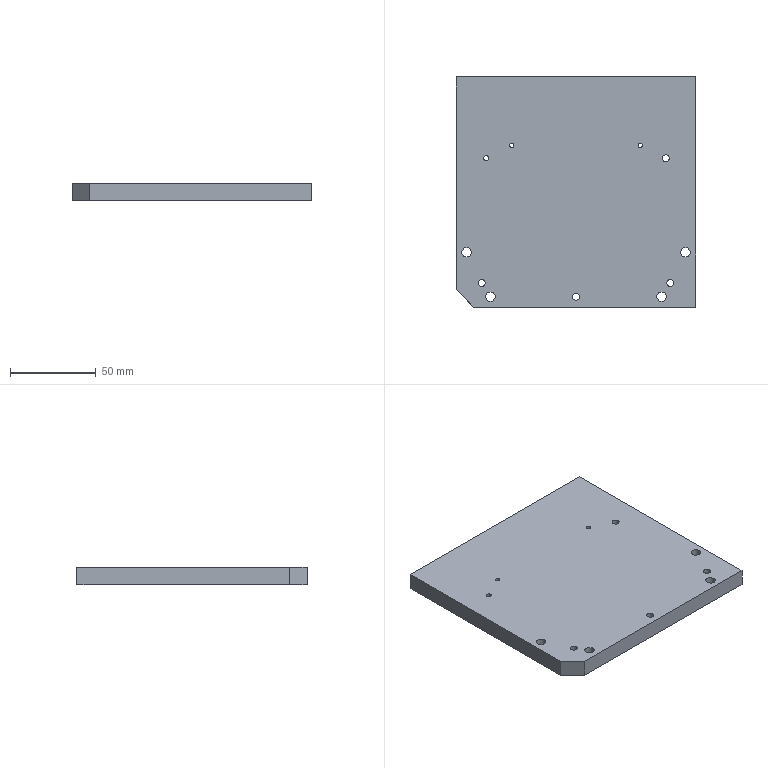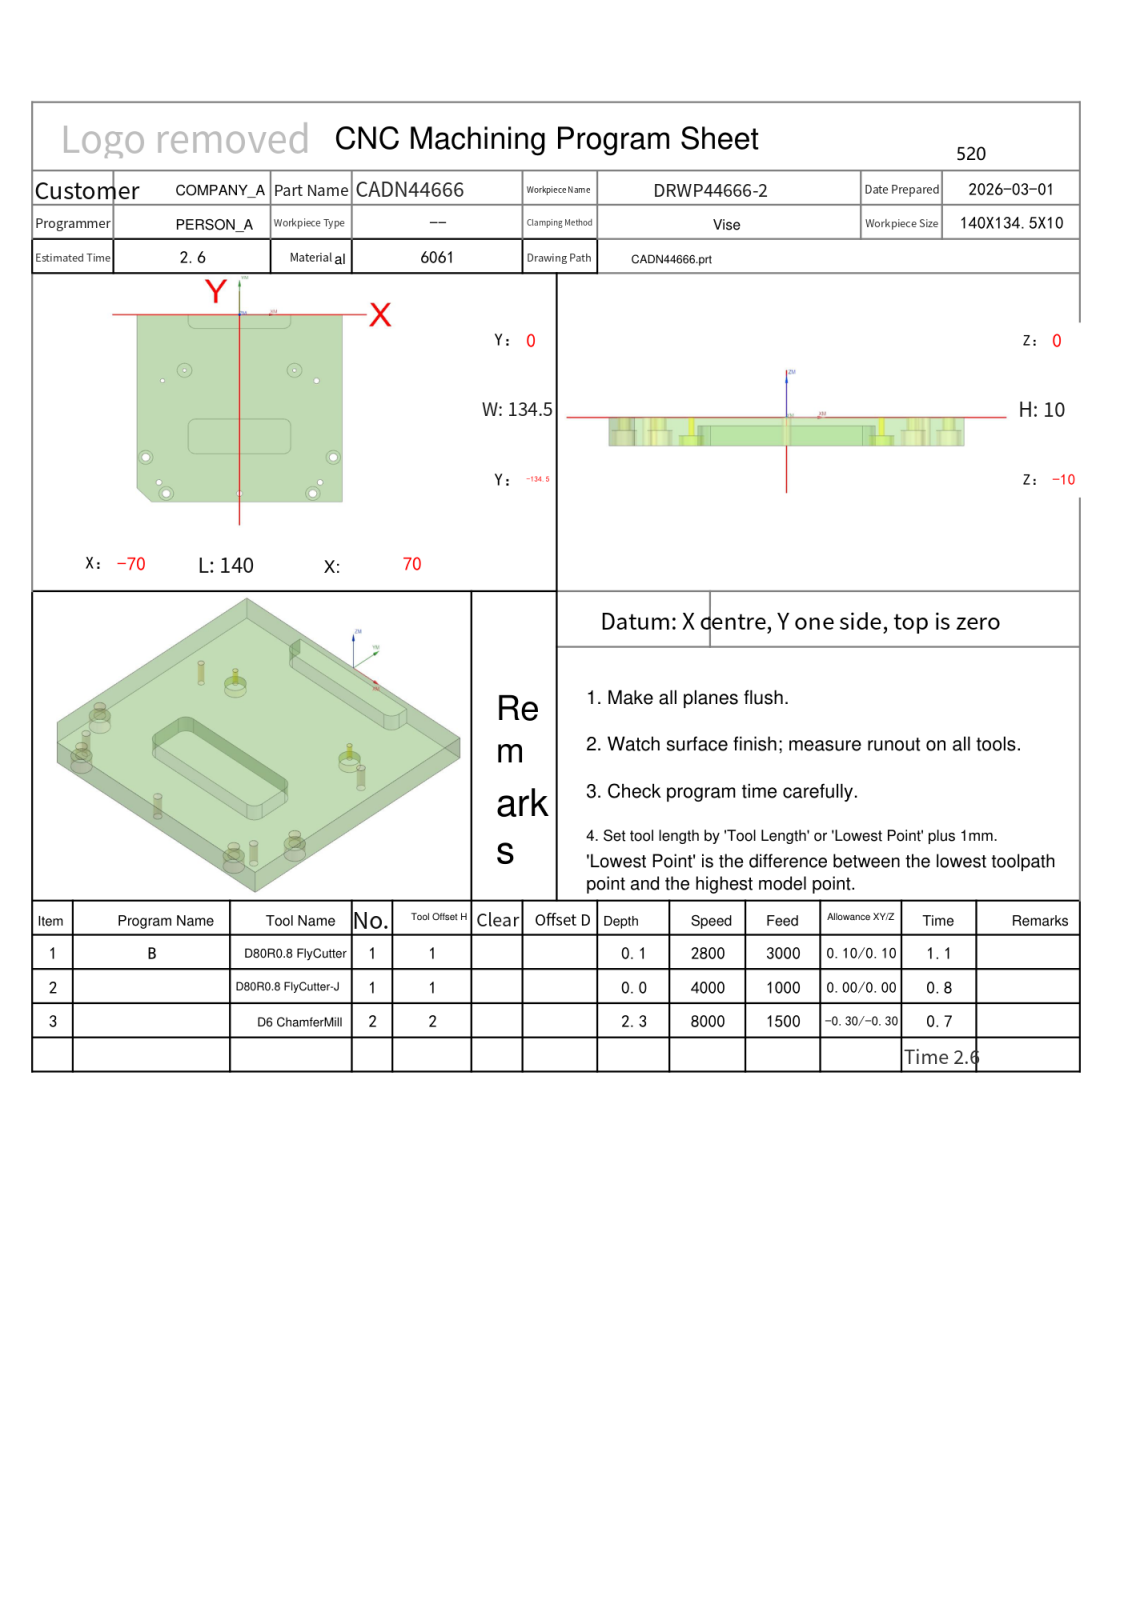NC program | NX | posted by the shop | part box 140 x 134.5 x 10 mm
Whole program:
%
O0001
(Machine time: 3.13 MIN)
(===Total Tool:2===)
(T1=D80R0.8 FlyCutter D=80.  R=0.8  D-  H01 Z=0.    )
(T2=D6 ChamferMill   D=6.   R=0.   D-  H02 Z=-2.3  )
G80 G90 G17 G49 G40
G91 G28 Z0
M01
N1 T01 M06
(D80R0.8 FlyCutter  D=80. R=0.8 H=01 ce=0.10 di=0.10)
G00 G90 G54 X-122.097 Y-23.903 M03 S2800
G43 H01 Z50.
M08
Z3.525
G01 Z1.525 F3000.
X-110.097
X102.897
G02 X110.097 Y-31.103 I0.0 J-7.2
G01 Y-55.57
G02 X102.097 Y-63.57 I-8. J0.0
G01 X-102.897
G03 X-110.097 Y-70.77 I0.0 J-7.2
G01 Y-95.237
G03 X-102.097 Y-103.237 I8. J0.0
G01 X110.097
X122.097
Z3.525
G00 X-122.097 Y-23.903
Z3.05
G01 Z1.05
X-110.097
X102.897
G02 X110.097 Y-31.103 I0.0 J-7.2
G01 Y-55.57
G02 X102.097 Y-63.57 I-8. J0.0
G01 X-102.897
G03 X-110.097 Y-70.77 I0.0 J-7.2
G01 Y-95.237
G03 X-102.097 Y-103.237 I8. J0.0
G01 X110.097
X122.097
Z3.05
G00 X-122.097 Y-23.903
Z2.575
G01 Z.575
X-110.097
X102.897
G02 X110.097 Y-31.103 I0.0 J-7.2
G01 Y-55.57
G02 X102.097 Y-63.57 I-8. J0.0
G01 X-102.897
G03 X-110.097 Y-70.77 I0.0 J-7.2
G01 Y-95.237
G03 X-102.097 Y-103.237 I8. J0.0
G01 X110.097
X122.097
Z2.575
G00 X-122.097 Y-23.903
Z2.1
G01 Z.1
X-110.097
X102.897
G02 X110.097 Y-31.103 I0.0 J-7.2
G01 Y-55.57
G02 X102.097 Y-63.57 I-8. J0.0
G01 X-102.897
G03 X-110.097 Y-70.77 I0.0 J-7.2
G01 Y-95.237
G03 X-102.097 Y-103.237 I8. J0.0
G01 X110.097
X122.097
Z2.1
G00 Z50.
G91 G28 Z0.0
M05
M09
G91 G28 Z0.0
M01
N2 T01 M06
(D80R0.8 FlyCutter-J  D=80. R=0.8 H=01 ce=0.00 di=0.00)
G00 G90 G54 X-121.999 Y-24.001 M03 S4000
G43 H01 Z50.
M08
Z2.
G01 Z0.0 F1000.
X-109.999
X102.799
G02 X109.999 Y-31.201 I0.0 J-7.2
G01 Y-55.57
G02 X101.999 Y-63.57 I-8. J0.0
G01 X-102.799
G03 X-109.999 Y-70.77 I0.0 J-7.2
G01 Y-95.139
G03 X-101.999 Y-103.139 I8. J0.0
G01 X109.999
X121.999
Z2.
G00 Z50.
G91 G28 Z0.0
M05
M09
G91 G28 Z0.0
M01
N3 T02 M06
(D6 ChamferMill  D=6. R=0. H=02 ce=0.00 di=0.00)
G00 G90 G54 X37.5 Y-40. M03 S8000
G43 H02 Z50.
M08
G98 G81 X37.5 Y-40. Z-1.75 R3. F1000.
X-37.5
G80
G00 Z50.
G00 G90 X-52.5 Y-47.5 M03 S8000
Z50.
G98 G81 X-52.5 Y-47.5 Z-1.8 R3. F1000.
G80
G00 Z50.
G00 G90 X52.5 Y-47.5 M03 S8000
Z50.
G98 G81 X52.5 Y-47.5 Z-2.3 R3. F1000.
X55. Y-120.5
X0.0 Y-128.5
X-55. Y-120.5
G80
G00 Z50.
G00 G90 X64.065 Y-103.147 M03 S8000
Z50.
Z-.9
G01 Z-1.4 F1200.
X64.15 Y-104.
G03 X65.65 Y-102.5 I0.0 J1.5
X64. Y-100.85 I-1.65 J0.0
X62.35 Y-102.5 I0.0 J-1.65
X64. Y-104.15 I1.65 J0.0
X65.65 Y-102.5 I0.0 J1.65
X64.15 Y-101. I-1.5 J0.0
G01 X64.065 Y-101.853
Z-.9
G00 Z50.
X50.065 Y-129.147
Z-.9
G01 Z-1.4
X50.15 Y-130.
G03 X51.65 Y-128.5 I0.0 J1.5
X50. Y-126.85 I-1.65 J0.0
X48.35 Y-128.5 I0.0 J-1.65
X50. Y-130.15 I1.65 J0.0
X51.65 Y-128.5 I0.0 J1.65
X50.15 Y-127. I-1.5 J0.0
G01 X50.065 Y-127.853
Z-.9
G00 Z50.
X-49.935 Y-129.147
Z-.9
G01 Z-1.4
X-49.85 Y-130.
G03 X-48.35 Y-128.5 I0.0 J1.5
X-50. Y-126.85 I-1.65 J0.0
X-51.65 Y-128.5 I0.0 J-1.65
X-50. Y-130.15 I1.65 J0.0
X-48.35 Y-128.5 I0.0 J1.65
X-49.85 Y-127. I-1.5 J0.0
G01 X-49.935 Y-127.853
Z-.9
G00 Z50.
X-63.935 Y-103.147
Z-.9
G01 Z-1.4
X-63.85 Y-104.
G03 X-62.35 Y-102.5 I0.0 J1.5
X-64. Y-100.85 I-1.65 J0.0
X-65.65 Y-102.5 I0.0 J-1.65
X-64. Y-104.15 I1.65 J0.0
X-62.35 Y-102.5 I0.0 J1.65
X-63.85 Y-101. I-1.5 J0.0
G01 X-63.935 Y-101.853
Z-.9
G00 Z50.
G00 G90 X-.386 Y1.227 M03 S6500
Z50.
Z.172
G01 Z-1.2 F1500.
G03 X-.1 Y1.027 I1.286 J1.532
G01 X-.054 Y.997
X0.0 Y1.
X70.
G02 X71. Y0.0 I0.0 J-1.
G01 Y-134.5
G02 X70. Y-135.5 I-1. J0.0
G01 X-60.
X-60.259 Y-135.466
X-60.5 Y-135.366
X-60.707 Y-135.207
X-70.707 Y-125.207
X-70.866 Y-125.
X-70.966 Y-124.759
X-71. Y-124.5
Y0.0
G02 X-70. Y1. I1. J0.0
G01 X0.0
X.054 Y.997
X.1 Y1.027
G03 X.386 Y1.227 I-1. J1.732
G01 Z.172
G00 Z10.
X-52.156 Y-47.919
Z.447
G01 Z-1.2
G03 X-52.009 Y-47.603 I-1.732 J1.
G01 X-51.988 Y-47.553
X-52. Y-47.5
G03 X-52.5 Y-47. I-.5 J0.0
X-53. Y-47.5 I0.0 J-.5
X-52.5 Y-48. I.5 J0.0
X-52. Y-47.5 I0.0 J.5
G01 X-51.988 Y-47.447
X-52.009 Y-47.397
G03 X-52.156 Y-47.081 I-1.879 J-.684
G01 Z.447
G00 Z10.
X-62.435 Y-102.907
Z.27
G01 Z-1.2
G03 X-62.266 Y-102.602 I-1.658 J1.118
G01 X-62.241 Y-102.554
X-62.25 Y-102.5
G03 X-64. Y-100.75 I-1.75 J0.0
X-65.75 Y-102.5 I0.0 J-1.75
X-64. Y-104.25 I1.75 J0.0
X-62.25 Y-102.5 I0.0 J1.75
G01 X-62.241 Y-102.446
X-62.266 Y-102.398
G03 X-62.435 Y-102.093 I-1.827 J-.813
G01 Z.27
G00 Z10.
X-54.174 Y-120.912
Z.33
G01 Z-1.2
G03 X-54.014 Y-120.603 I-1.687 J1.075
G01 X-53.99 Y-120.554
X-54. Y-120.5
G03 X-55. Y-119.5 I-1. J0.0
X-56. Y-120.5 I0.0 J-1.
X-55. Y-121.5 I1. J0.0
X-54. Y-120.5 I0.0 J1.
G01 X-53.99 Y-120.446
X-54.014 Y-120.397
G03 X-54.174 Y-120.088 I-1.848 J-.765
G01 Z.33
G00 Z2.55
X-48.435 Y-128.907
Z.27
G01 Z-1.2
G03 X-48.266 Y-128.602 I-1.658 J1.118
G01 X-48.241 Y-128.554
X-48.25 Y-128.5
G03 X-50. Y-126.75 I-1.75 J0.0
X-51.75 Y-128.5 I0.0 J-1.75
X-50. Y-130.25 I1.75 J0.0
X-48.25 Y-128.5 I0.0 J1.75
G01 X-48.241 Y-128.446
X-48.266 Y-128.398
G03 X-48.435 Y-128.093 I-1.827 J-.813
G01 Z.27
G00 Z10.
X.826 Y-128.912
Z.33
G01 Z-1.2
G03 X.986 Y-128.603 I-1.687 J1.075
G01 X1.01 Y-128.554
X1. Y-128.5
G03 X0.0 Y-127.5 I-1. J0.0
X-1. Y-128.5 I0.0 J-1.
X0.0 Y-129.5 I1. J0.0
X1. Y-128.5 I0.0 J1.
G01 X1.01 Y-128.446
X.986 Y-128.397
G03 X.826 Y-128.088 I-1.848 J-.765
G01 Z.33
G00 Z10.
X51.565 Y-128.907
Z.27
G01 Z-1.2
G03 X51.734 Y-128.602 I-1.658 J1.118
G01 X51.759 Y-128.554
X51.75 Y-128.5
G03 X50. Y-126.75 I-1.75 J0.0
X48.25 Y-128.5 I0.0 J-1.75
X50. Y-130.25 I1.75 J0.0
X51.75 Y-128.5 I0.0 J1.75
G01 X51.759 Y-128.446
X51.734 Y-128.398
G03 X51.565 Y-128.093 I-1.827 J-.813
G01 Z.27
G00 Z2.55
X55.826 Y-120.912
Z.33
G01 Z-1.2
G03 X55.986 Y-120.603 I-1.687 J1.075
G01 X56.01 Y-120.554
X56. Y-120.5
G03 X55. Y-119.5 I-1. J0.0
X54. Y-120.5 I0.0 J-1.
X55. Y-121.5 I1. J0.0
X56. Y-120.5 I0.0 J1.
G01 X56.01 Y-120.446
X55.986 Y-120.397
G03 X55.826 Y-120.088 I-1.848 J-.765
G01 Z.33
G00 Z10.
X65.565 Y-102.907
Z.27
G01 Z-1.2
G03 X65.734 Y-102.602 I-1.658 J1.118
G01 X65.759 Y-102.554
X65.75 Y-102.5
G03 X64. Y-100.75 I-1.75 J0.0
X62.25 Y-102.5 I0.0 J-1.75
X64. Y-104.25 I1.75 J0.0
X65.75 Y-102.5 I0.0 J1.75
G01 X65.759 Y-102.446
X65.734 Y-102.398
G03 X65.565 Y-102.093 I-1.827 J-.813
G01 Z.27
G00 Z10.
X53.326 Y-47.912
Z.33
G01 Z-1.2
G03 X53.486 Y-47.603 I-1.687 J1.075
G01 X53.51 Y-47.554
X53.5 Y-47.5
G03 X52.5 Y-46.5 I-1. J0.0
X51.5 Y-47.5 I0.0 J-1.
X52.5 Y-48.5 I1. J0.0
X53.5 Y-47.5 I0.0 J1.
G01 X53.51 Y-47.446
X53.486 Y-47.397
G03 X53.326 Y-47.088 I-1.848 J-.765
G01 Z.33
G00 Z50.
M05
M09
G91 G28 Z0.0
G91 G28 Y0.0
M30
%